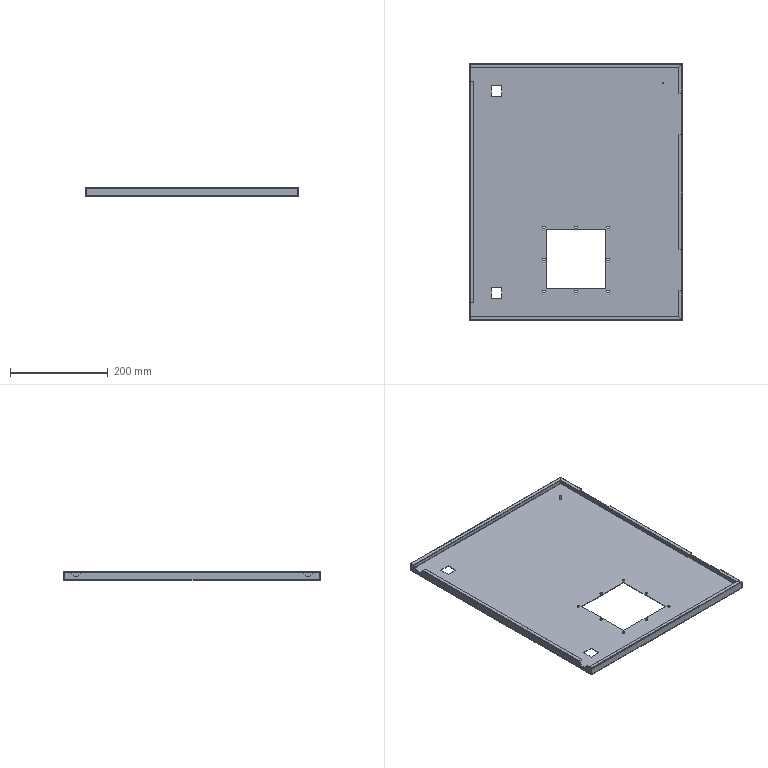Part | STEP file | right door panel 2 | 1 solid | 165 faces | box 435.5 x 525.8 x 17 mm | volume 303156 mm3 | plane 113 | cylinder 46 | spline 6 | commonest cylinder face diameters 5 x16 0.02 x10 2.42 x10 2 x4 4 x4 3 x2